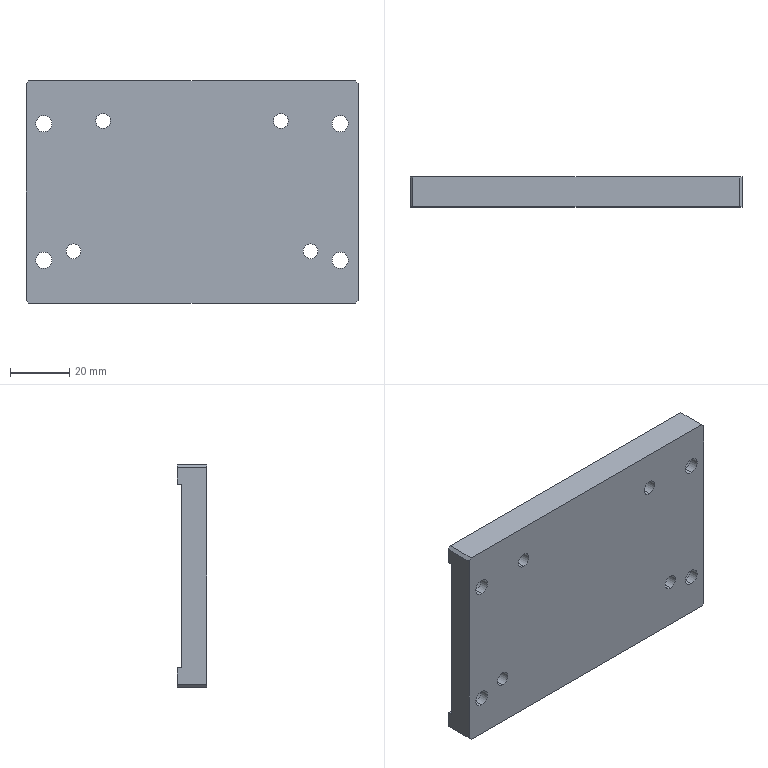Part | NX | features BREP 1 | 1 solid | 42 faces | box 112 x 10 x 75 mm | volume 70883 mm3 | cylinder 24 | plane 18 | commonest cylinder face diameters 5 x8 5.5 x8 10 x8
STEP:
#1=CARTESIAN_POINT('',(-40.,-5.,-22.5));
#2=VERTEX_POINT('',#1);
#3=CARTESIAN_POINT('',(-40.,-5.,-17.5));
#4=VERTEX_POINT('',#3);
#5=CARTESIAN_POINT('',(-40.,-5.,-20.));
#6=DIRECTION('',(0.,1.,0.));
#7=DIRECTION('',(0.,0.,1.));
#8=AXIS2_PLACEMENT_3D('',#5,#6,#7);
#9=CIRCLE('',#8,2.5);
#10=EDGE_CURVE('',#2,#4,#9,.T.);
#11=ORIENTED_EDGE('',*,*,#10,.F.);
#12=CARTESIAN_POINT('',(-40.,3.5,-22.5));
#13=VERTEX_POINT('',#12);
#14=CARTESIAN_POINT('',(-40.,3.5,-22.5));
#15=DIRECTION('',(0.,1.,0.));
#16=VECTOR('',#15,1000.);
#17=LINE('',#14,#16);
#18=EDGE_CURVE('',#13,#2,#17,.F.);
#19=ORIENTED_EDGE('',*,*,#18,.F.);
#20=CARTESIAN_POINT('',(-40.,3.5,-17.5));
#21=VERTEX_POINT('',#20);
#22=CARTESIAN_POINT('',(-40.,3.5,-20.));
#23=DIRECTION('',(0.,1.,0.));
#24=DIRECTION('',(0.,0.,1.));
#25=AXIS2_PLACEMENT_3D('',#22,#23,#24);
#26=CIRCLE('',#25,2.5);
#27=EDGE_CURVE('',#13,#21,#26,.T.);
#28=ORIENTED_EDGE('',*,*,#27,.T.);
#29=CARTESIAN_POINT('',(-40.,3.5,-17.5));
#30=DIRECTION('',(0.,1.,0.));
#31=VECTOR('',#30,1000.);
#32=LINE('',#29,#31);
#33=EDGE_CURVE('',#21,#4,#32,.F.);
#34=ORIENTED_EDGE('',*,*,#33,.T.);
#35=EDGE_LOOP('',(#11,#19,#28,#34));
#36=FACE_BOUND('',#35,.T.);
#37=CARTESIAN_POINT('',(-40.,3.5,-20.));
#38=DIRECTION('',(0.,1.,0.));
#39=DIRECTION('',(0.,0.,1.));
#40=AXIS2_PLACEMENT_3D('',#37,#38,#39);
#41=CYLINDRICAL_SURFACE('',#40,2.5);
#42=ADVANCED_FACE('',(#36),#41,.F.);
#43=CARTESIAN_POINT('',(40.,-5.,-22.5));
#44=VERTEX_POINT('',#43);
#45=CARTESIAN_POINT('',(40.,-5.,-17.5));
#46=VERTEX_POINT('',#45);
#47=CARTESIAN_POINT('',(40.,-5.,-20.));
#48=DIRECTION('',(0.,1.,0.));
#49=DIRECTION('',(0.,0.,1.));
#50=AXIS2_PLACEMENT_3D('',#47,#48,#49);
#51=CIRCLE('',#50,2.5);
#52=EDGE_CURVE('',#44,#46,#51,.T.);
#53=ORIENTED_EDGE('',*,*,#52,.F.);
#54=CARTESIAN_POINT('',(40.,3.5,-22.5));
#55=VERTEX_POINT('',#54);
#56=CARTESIAN_POINT('',(40.,3.5,-22.5));
#57=DIRECTION('',(0.,1.,0.));
#58=VECTOR('',#57,1000.);
#59=LINE('',#56,#58);
#60=EDGE_CURVE('',#55,#44,#59,.F.);
#61=ORIENTED_EDGE('',*,*,#60,.F.);
#62=CARTESIAN_POINT('',(40.,3.5,-17.5));
#63=VERTEX_POINT('',#62);
#64=CARTESIAN_POINT('',(40.,3.5,-20.));
#65=DIRECTION('',(0.,1.,0.));
#66=DIRECTION('',(0.,0.,1.));
#67=AXIS2_PLACEMENT_3D('',#64,#65,#66);
#68=CIRCLE('',#67,2.5);
#69=EDGE_CURVE('',#55,#63,#68,.T.);
#70=ORIENTED_EDGE('',*,*,#69,.T.);
#71=CARTESIAN_POINT('',(40.,3.5,-17.5));
#72=DIRECTION('',(0.,1.,0.));
#73=VECTOR('',#72,1000.);
#74=LINE('',#71,#73);
#75=EDGE_CURVE('',#63,#46,#74,.F.);
#76=ORIENTED_EDGE('',*,*,#75,.T.);
#77=EDGE_LOOP('',(#53,#61,#70,#76));
#78=FACE_BOUND('',#77,.T.);
#79=CARTESIAN_POINT('',(40.,3.5,-20.));
#80=DIRECTION('',(0.,1.,0.));
#81=DIRECTION('',(0.,0.,1.));
#82=AXIS2_PLACEMENT_3D('',#79,#80,#81);
#83=CYLINDRICAL_SURFACE('',#82,2.5);
#84=ADVANCED_FACE('',(#78),#83,.F.);
#85=CARTESIAN_POINT('',(-30.,-5.,21.5));
#86=VERTEX_POINT('',#85);
#87=CARTESIAN_POINT('',(-30.,-5.,26.5));
#88=VERTEX_POINT('',#87);
#89=CARTESIAN_POINT('',(-30.,-5.,24.));
#90=DIRECTION('',(0.,1.,0.));
#91=DIRECTION('',(0.,0.,1.));
#92=AXIS2_PLACEMENT_3D('',#89,#90,#91);
#93=CIRCLE('',#92,2.5);
#94=EDGE_CURVE('',#86,#88,#93,.T.);
#95=ORIENTED_EDGE('',*,*,#94,.F.);
#96=CARTESIAN_POINT('',(-30.,3.5,21.5));
#97=VERTEX_POINT('',#96);
#98=CARTESIAN_POINT('',(-30.,3.5,21.5));
#99=DIRECTION('',(0.,1.,0.));
#100=VECTOR('',#99,1000.);
#101=LINE('',#98,#100);
#102=EDGE_CURVE('',#97,#86,#101,.F.);
#103=ORIENTED_EDGE('',*,*,#102,.F.);
#104=CARTESIAN_POINT('',(-30.,3.5,26.5));
#105=VERTEX_POINT('',#104);
#106=CARTESIAN_POINT('',(-30.,3.5,24.));
#107=DIRECTION('',(0.,1.,0.));
#108=DIRECTION('',(0.,0.,1.));
#109=AXIS2_PLACEMENT_3D('',#106,#107,#108);
#110=CIRCLE('',#109,2.5);
#111=EDGE_CURVE('',#97,#105,#110,.T.);
#112=ORIENTED_EDGE('',*,*,#111,.T.);
#113=CARTESIAN_POINT('',(-30.,3.5,26.5));
#114=DIRECTION('',(0.,1.,0.));
#115=VECTOR('',#114,1000.);
#116=LINE('',#113,#115);
#117=EDGE_CURVE('',#105,#88,#116,.F.);
#118=ORIENTED_EDGE('',*,*,#117,.T.);
#119=EDGE_LOOP('',(#95,#103,#112,#118));
#120=FACE_BOUND('',#119,.T.);
#121=CARTESIAN_POINT('',(-30.,3.5,24.));
#122=DIRECTION('',(0.,1.,0.));
#123=DIRECTION('',(0.,0.,1.));
#124=AXIS2_PLACEMENT_3D('',#121,#122,#123);
#125=CYLINDRICAL_SURFACE('',#124,2.5);
#126=ADVANCED_FACE('',(#120),#125,.F.);
#127=CARTESIAN_POINT('',(30.,-5.,21.5));
#128=VERTEX_POINT('',#127);
#129=CARTESIAN_POINT('',(30.,-5.,26.5));
#130=VERTEX_POINT('',#129);
#131=CARTESIAN_POINT('',(30.,-5.,24.));
#132=DIRECTION('',(0.,1.,0.));
#133=DIRECTION('',(0.,0.,1.));
#134=AXIS2_PLACEMENT_3D('',#131,#132,#133);
#135=CIRCLE('',#134,2.5);
#136=EDGE_CURVE('',#128,#130,#135,.T.);
#137=ORIENTED_EDGE('',*,*,#136,.F.);
#138=CARTESIAN_POINT('',(30.,3.5,21.5));
#139=VERTEX_POINT('',#138);
#140=CARTESIAN_POINT('',(30.,3.5,21.5));
#141=DIRECTION('',(0.,1.,0.));
#142=VECTOR('',#141,1000.);
#143=LINE('',#140,#142);
#144=EDGE_CURVE('',#139,#128,#143,.F.);
#145=ORIENTED_EDGE('',*,*,#144,.F.);
#146=CARTESIAN_POINT('',(30.,3.5,26.5));
#147=VERTEX_POINT('',#146);
#148=CARTESIAN_POINT('',(30.,3.5,24.));
#149=DIRECTION('',(0.,1.,0.));
#150=DIRECTION('',(0.,0.,1.));
#151=AXIS2_PLACEMENT_3D('',#148,#149,#150);
#152=CIRCLE('',#151,2.5);
#153=EDGE_CURVE('',#139,#147,#152,.T.);
#154=ORIENTED_EDGE('',*,*,#153,.T.);
#155=CARTESIAN_POINT('',(30.,3.5,26.5));
#156=DIRECTION('',(0.,1.,0.));
#157=VECTOR('',#156,1000.);
#158=LINE('',#155,#157);
#159=EDGE_CURVE('',#147,#130,#158,.F.);
#160=ORIENTED_EDGE('',*,*,#159,.T.);
#161=EDGE_LOOP('',(#137,#145,#154,#160));
#162=FACE_BOUND('',#161,.T.);
#163=CARTESIAN_POINT('',(30.,3.5,24.));
#164=DIRECTION('',(0.,1.,0.));
#165=DIRECTION('',(0.,0.,1.));
#166=AXIS2_PLACEMENT_3D('',#163,#164,#165);
#167=CYLINDRICAL_SURFACE('',#166,2.5);
#168=ADVANCED_FACE('',(#162),#167,.F.);
#169=CARTESIAN_POINT('',(-50.,-5.,20.25));
#170=VERTEX_POINT('',#169);
#171=CARTESIAN_POINT('',(-50.,-5.,25.75));
#172=VERTEX_POINT('',#171);
#173=CARTESIAN_POINT('',(-50.,-5.,23.));
#174=DIRECTION('',(0.,1.,0.));
#175=DIRECTION('',(0.,0.,1.));
#176=AXIS2_PLACEMENT_3D('',#173,#174,#175);
#177=CIRCLE('',#176,2.75);
#178=EDGE_CURVE('',#170,#172,#177,.T.);
#179=ORIENTED_EDGE('',*,*,#178,.F.);
#180=CARTESIAN_POINT('',(-50.,-2.,20.25));
#181=VERTEX_POINT('',#180);
#182=CARTESIAN_POINT('',(-50.,5.,20.25));
#183=DIRECTION('',(0.,1.,0.));
#184=VECTOR('',#183,1000.);
#185=LINE('',#182,#184);
#186=EDGE_CURVE('',#181,#170,#185,.F.);
#187=ORIENTED_EDGE('',*,*,#186,.F.);
#188=CARTESIAN_POINT('',(-50.,-2.,25.75));
#189=VERTEX_POINT('',#188);
#190=CARTESIAN_POINT('',(-50.,-2.,23.));
#191=DIRECTION('',(0.,1.,0.));
#192=DIRECTION('',(0.,0.,1.));
#193=AXIS2_PLACEMENT_3D('',#190,#191,#192);
#194=CIRCLE('',#193,2.75);
#195=EDGE_CURVE('',#181,#189,#194,.T.);
#196=ORIENTED_EDGE('',*,*,#195,.T.);
#197=CARTESIAN_POINT('',(-50.,5.,25.75));
#198=DIRECTION('',(0.,1.,0.));
#199=VECTOR('',#198,1000.);
#200=LINE('',#197,#199);
#201=EDGE_CURVE('',#189,#172,#200,.F.);
#202=ORIENTED_EDGE('',*,*,#201,.T.);
#203=EDGE_LOOP('',(#179,#187,#196,#202));
#204=FACE_BOUND('',#203,.T.);
#205=CARTESIAN_POINT('',(-50.,5.,23.));
#206=DIRECTION('',(0.,1.,0.));
#207=DIRECTION('',(0.,0.,1.));
#208=AXIS2_PLACEMENT_3D('',#205,#206,#207);
#209=CYLINDRICAL_SURFACE('',#208,2.75);
#210=ADVANCED_FACE('',(#204),#209,.F.);
#211=CARTESIAN_POINT('',(-50.,-5.,-25.75));
#212=VERTEX_POINT('',#211);
#213=CARTESIAN_POINT('',(-50.,-5.,-20.25));
#214=VERTEX_POINT('',#213);
#215=CARTESIAN_POINT('',(-50.,-5.,-23.));
#216=DIRECTION('',(0.,1.,0.));
#217=DIRECTION('',(0.,0.,1.));
#218=AXIS2_PLACEMENT_3D('',#215,#216,#217);
#219=CIRCLE('',#218,2.75);
#220=EDGE_CURVE('',#212,#214,#219,.T.);
#221=ORIENTED_EDGE('',*,*,#220,.F.);
#222=CARTESIAN_POINT('',(-50.,-2.,-25.75));
#223=VERTEX_POINT('',#222);
#224=CARTESIAN_POINT('',(-50.,5.,-25.75));
#225=DIRECTION('',(0.,1.,0.));
#226=VECTOR('',#225,1000.);
#227=LINE('',#224,#226);
#228=EDGE_CURVE('',#223,#212,#227,.F.);
#229=ORIENTED_EDGE('',*,*,#228,.F.);
#230=CARTESIAN_POINT('',(-50.,-2.,-20.25));
#231=VERTEX_POINT('',#230);
#232=CARTESIAN_POINT('',(-50.,-2.,-23.));
#233=DIRECTION('',(0.,1.,0.));
#234=DIRECTION('',(0.,0.,1.));
#235=AXIS2_PLACEMENT_3D('',#232,#233,#234);
#236=CIRCLE('',#235,2.75);
#237=EDGE_CURVE('',#223,#231,#236,.T.);
#238=ORIENTED_EDGE('',*,*,#237,.T.);
#239=CARTESIAN_POINT('',(-50.,5.,-20.25));
#240=DIRECTION('',(0.,1.,0.));
#241=VECTOR('',#240,1000.);
#242=LINE('',#239,#241);
#243=EDGE_CURVE('',#231,#214,#242,.F.);
#244=ORIENTED_EDGE('',*,*,#243,.T.);
#245=EDGE_LOOP('',(#221,#229,#238,#244));
#246=FACE_BOUND('',#245,.T.);
#247=CARTESIAN_POINT('',(-50.,5.,-23.));
#248=DIRECTION('',(0.,1.,0.));
#249=DIRECTION('',(0.,0.,1.));
#250=AXIS2_PLACEMENT_3D('',#247,#248,#249);
#251=CYLINDRICAL_SURFACE('',#250,2.75);
#252=ADVANCED_FACE('',(#246),#251,.F.);
#253=CARTESIAN_POINT('',(50.,-5.,-25.75));
#254=VERTEX_POINT('',#253);
#255=CARTESIAN_POINT('',(50.,-5.,-20.25));
#256=VERTEX_POINT('',#255);
#257=CARTESIAN_POINT('',(50.,-5.,-23.));
#258=DIRECTION('',(0.,1.,0.));
#259=DIRECTION('',(0.,0.,1.));
#260=AXIS2_PLACEMENT_3D('',#257,#258,#259);
#261=CIRCLE('',#260,2.75);
#262=EDGE_CURVE('',#254,#256,#261,.T.);
#263=ORIENTED_EDGE('',*,*,#262,.F.);
#264=CARTESIAN_POINT('',(50.,-2.,-25.75));
#265=VERTEX_POINT('',#264);
#266=CARTESIAN_POINT('',(50.,5.,-25.75));
#267=DIRECTION('',(0.,1.,0.));
#268=VECTOR('',#267,1000.);
#269=LINE('',#266,#268);
#270=EDGE_CURVE('',#265,#254,#269,.F.);
#271=ORIENTED_EDGE('',*,*,#270,.F.);
#272=CARTESIAN_POINT('',(50.,-2.,-20.25));
#273=VERTEX_POINT('',#272);
#274=CARTESIAN_POINT('',(50.,-2.,-23.));
#275=DIRECTION('',(0.,1.,0.));
#276=DIRECTION('',(0.,0.,1.));
#277=AXIS2_PLACEMENT_3D('',#274,#275,#276);
#278=CIRCLE('',#277,2.75);
#279=EDGE_CURVE('',#265,#273,#278,.T.);
#280=ORIENTED_EDGE('',*,*,#279,.T.);
#281=CARTESIAN_POINT('',(50.,5.,-20.25));
#282=DIRECTION('',(0.,1.,0.));
#283=VECTOR('',#282,1000.);
#284=LINE('',#281,#283);
#285=EDGE_CURVE('',#273,#256,#284,.F.);
#286=ORIENTED_EDGE('',*,*,#285,.T.);
#287=EDGE_LOOP('',(#263,#271,#280,#286));
#288=FACE_BOUND('',#287,.T.);
#289=CARTESIAN_POINT('',(50.,5.,-23.));
#290=DIRECTION('',(0.,1.,0.));
#291=DIRECTION('',(0.,0.,1.));
#292=AXIS2_PLACEMENT_3D('',#289,#290,#291);
#293=CYLINDRICAL_SURFACE('',#292,2.75);
#294=ADVANCED_FACE('',(#288),#293,.F.);
#295=CARTESIAN_POINT('',(50.,-5.,20.25));
#296=VERTEX_POINT('',#295);
#297=CARTESIAN_POINT('',(50.,-5.,25.75));
#298=VERTEX_POINT('',#297);
#299=CARTESIAN_POINT('',(50.,-5.,23.));
#300=DIRECTION('',(0.,1.,0.));
#301=DIRECTION('',(0.,0.,1.));
#302=AXIS2_PLACEMENT_3D('',#299,#300,#301);
#303=CIRCLE('',#302,2.75);
#304=EDGE_CURVE('',#296,#298,#303,.T.);
#305=ORIENTED_EDGE('',*,*,#304,.F.);
#306=CARTESIAN_POINT('',(50.,-2.,20.25));
#307=VERTEX_POINT('',#306);
#308=CARTESIAN_POINT('',(50.,5.,20.25));
#309=DIRECTION('',(0.,1.,0.));
#310=VECTOR('',#309,1000.);
#311=LINE('',#308,#310);
#312=EDGE_CURVE('',#307,#296,#311,.F.);
#313=ORIENTED_EDGE('',*,*,#312,.F.);
#314=CARTESIAN_POINT('',(50.,-2.,25.75));
#315=VERTEX_POINT('',#314);
#316=CARTESIAN_POINT('',(50.,-2.,23.));
#317=DIRECTION('',(0.,1.,0.));
#318=DIRECTION('',(0.,0.,1.));
#319=AXIS2_PLACEMENT_3D('',#316,#317,#318);
#320=CIRCLE('',#319,2.75);
#321=EDGE_CURVE('',#307,#315,#320,.T.);
#322=ORIENTED_EDGE('',*,*,#321,.T.);
#323=CARTESIAN_POINT('',(50.,5.,25.75));
#324=DIRECTION('',(0.,1.,0.));
#325=VECTOR('',#324,1000.);
#326=LINE('',#323,#325);
#327=EDGE_CURVE('',#315,#298,#326,.F.);
#328=ORIENTED_EDGE('',*,*,#327,.T.);
#329=EDGE_LOOP('',(#305,#313,#322,#328));
#330=FACE_BOUND('',#329,.T.);
#331=CARTESIAN_POINT('',(50.,5.,23.));
#332=DIRECTION('',(0.,1.,0.));
#333=DIRECTION('',(0.,0.,1.));
#334=AXIS2_PLACEMENT_3D('',#331,#332,#333);
#335=CYLINDRICAL_SURFACE('',#334,2.75);
#336=ADVANCED_FACE('',(#330),#335,.F.);
#337=CARTESIAN_POINT('',(-50.,-2.,18.));
#338=VERTEX_POINT('',#337);
#339=CARTESIAN_POINT('',(-50.,-2.,28.));
#340=VERTEX_POINT('',#339);
#341=CARTESIAN_POINT('',(-50.,-2.,23.));
#342=DIRECTION('',(0.,1.,0.));
#343=DIRECTION('',(0.,0.,1.));
#344=AXIS2_PLACEMENT_3D('',#341,#342,#343);
#345=CIRCLE('',#344,5.);
#346=EDGE_CURVE('',#338,#340,#345,.T.);
#347=ORIENTED_EDGE('',*,*,#346,.F.);
#348=CARTESIAN_POINT('',(-50.,3.5,18.));
#349=VERTEX_POINT('',#348);
#350=CARTESIAN_POINT('',(-50.,5.,18.));
#351=DIRECTION('',(0.,1.,0.));
#352=VECTOR('',#351,1000.);
#353=LINE('',#350,#352);
#354=EDGE_CURVE('',#349,#338,#353,.F.);
#355=ORIENTED_EDGE('',*,*,#354,.F.);
#356=CARTESIAN_POINT('',(-50.,3.5,28.));
#357=VERTEX_POINT('',#356);
#358=CARTESIAN_POINT('',(-50.,3.5,23.));
#359=DIRECTION('',(0.,-1.,0.));
#360=DIRECTION('',(0.,0.,1.));
#361=AXIS2_PLACEMENT_3D('',#358,#359,#360);
#362=CIRCLE('',#361,5.);
#363=EDGE_CURVE('',#357,#349,#362,.T.);
#364=ORIENTED_EDGE('',*,*,#363,.F.);
#365=CARTESIAN_POINT('',(-50.,5.,28.));
#366=DIRECTION('',(0.,1.,0.));
#367=VECTOR('',#366,1000.);
#368=LINE('',#365,#367);
#369=EDGE_CURVE('',#357,#340,#368,.F.);
#370=ORIENTED_EDGE('',*,*,#369,.T.);
#371=EDGE_LOOP('',(#347,#355,#364,#370));
#372=FACE_BOUND('',#371,.T.);
#373=CARTESIAN_POINT('',(-50.,5.,23.));
#374=DIRECTION('',(0.,1.,0.));
#375=DIRECTION('',(0.,0.,1.));
#376=AXIS2_PLACEMENT_3D('',#373,#374,#375);
#377=CYLINDRICAL_SURFACE('',#376,5.);
#378=ADVANCED_FACE('',(#372),#377,.F.);
#379=CARTESIAN_POINT('',(-50.,-2.,-28.));
#380=VERTEX_POINT('',#379);
#381=CARTESIAN_POINT('',(-50.,-2.,-18.));
#382=VERTEX_POINT('',#381);
#383=CARTESIAN_POINT('',(-50.,-2.,-23.));
#384=DIRECTION('',(0.,1.,0.));
#385=DIRECTION('',(0.,0.,1.));
#386=AXIS2_PLACEMENT_3D('',#383,#384,#385);
#387=CIRCLE('',#386,5.);
#388=EDGE_CURVE('',#380,#382,#387,.T.);
#389=ORIENTED_EDGE('',*,*,#388,.F.);
#390=CARTESIAN_POINT('',(-50.,3.5,-28.));
#391=VERTEX_POINT('',#390);
#392=CARTESIAN_POINT('',(-50.,5.,-28.));
#393=DIRECTION('',(0.,1.,0.));
#394=VECTOR('',#393,1000.);
#395=LINE('',#392,#394);
#396=EDGE_CURVE('',#391,#380,#395,.F.);
#397=ORIENTED_EDGE('',*,*,#396,.F.);
#398=CARTESIAN_POINT('',(-50.,3.5,-18.));
#399=VERTEX_POINT('',#398);
#400=CARTESIAN_POINT('',(-50.,3.5,-23.));
#401=DIRECTION('',(0.,-1.,0.));
#402=DIRECTION('',(0.,0.,1.));
#403=AXIS2_PLACEMENT_3D('',#400,#401,#402);
#404=CIRCLE('',#403,5.);
#405=EDGE_CURVE('',#399,#391,#404,.T.);
#406=ORIENTED_EDGE('',*,*,#405,.F.);
#407=CARTESIAN_POINT('',(-50.,5.,-18.));
#408=DIRECTION('',(0.,1.,0.));
#409=VECTOR('',#408,1000.);
#410=LINE('',#407,#409);
#411=EDGE_CURVE('',#399,#382,#410,.F.);
#412=ORIENTED_EDGE('',*,*,#411,.T.);
#413=EDGE_LOOP('',(#389,#397,#406,#412));
#414=FACE_BOUND('',#413,.T.);
#415=CARTESIAN_POINT('',(-50.,5.,-23.));
#416=DIRECTION('',(0.,1.,0.));
#417=DIRECTION('',(0.,0.,1.));
#418=AXIS2_PLACEMENT_3D('',#415,#416,#417);
#419=CYLINDRICAL_SURFACE('',#418,5.);
#420=ADVANCED_FACE('',(#414),#419,.F.);
#421=CARTESIAN_POINT('',(50.,-2.,-28.));
#422=VERTEX_POINT('',#421);
#423=CARTESIAN_POINT('',(50.,-2.,-18.));
#424=VERTEX_POINT('',#423);
#425=CARTESIAN_POINT('',(50.,-2.,-23.));
#426=DIRECTION('',(0.,1.,0.));
#427=DIRECTION('',(0.,0.,1.));
#428=AXIS2_PLACEMENT_3D('',#425,#426,#427);
#429=CIRCLE('',#428,5.);
#430=EDGE_CURVE('',#422,#424,#429,.T.);
#431=ORIENTED_EDGE('',*,*,#430,.F.);
#432=CARTESIAN_POINT('',(50.,3.5,-28.));
#433=VERTEX_POINT('',#432);
#434=CARTESIAN_POINT('',(50.,5.,-28.));
#435=DIRECTION('',(0.,1.,0.));
#436=VECTOR('',#435,1000.);
#437=LINE('',#434,#436);
#438=EDGE_CURVE('',#433,#422,#437,.F.);
#439=ORIENTED_EDGE('',*,*,#438,.F.);
#440=CARTESIAN_POINT('',(50.,3.5,-18.));
#441=VERTEX_POINT('',#440);
#442=CARTESIAN_POINT('',(50.,3.5,-23.));
#443=DIRECTION('',(0.,-1.,0.));
#444=DIRECTION('',(0.,0.,1.));
#445=AXIS2_PLACEMENT_3D('',#442,#443,#444);
#446=CIRCLE('',#445,5.);
#447=EDGE_CURVE('',#441,#433,#446,.T.);
#448=ORIENTED_EDGE('',*,*,#447,.F.);
#449=CARTESIAN_POINT('',(50.,5.,-18.));
#450=DIRECTION('',(0.,1.,0.));
#451=VECTOR('',#450,1000.);
#452=LINE('',#449,#451);
#453=EDGE_CURVE('',#441,#424,#452,.F.);
#454=ORIENTED_EDGE('',*,*,#453,.T.);
#455=EDGE_LOOP('',(#431,#439,#448,#454));
#456=FACE_BOUND('',#455,.T.);
#457=CARTESIAN_POINT('',(50.,5.,-23.));
#458=DIRECTION('',(0.,1.,0.));
#459=DIRECTION('',(0.,0.,1.));
#460=AXIS2_PLACEMENT_3D('',#457,#458,#459);
#461=CYLINDRICAL_SURFACE('',#460,5.);
#462=ADVANCED_FACE('',(#456),#461,.F.);
#463=CARTESIAN_POINT('',(50.,-2.,18.));
#464=VERTEX_POINT('',#463);
#465=CARTESIAN_POINT('',(50.,-2.,28.));
#466=VERTEX_POINT('',#465);
#467=CARTESIAN_POINT('',(50.,-2.,23.));
#468=DIRECTION('',(0.,1.,0.));
#469=DIRECTION('',(0.,0.,1.));
#470=AXIS2_PLACEMENT_3D('',#467,#468,#469);
#471=CIRCLE('',#470,5.);
#472=EDGE_CURVE('',#464,#466,#471,.T.);
#473=ORIENTED_EDGE('',*,*,#472,.F.);
#474=CARTESIAN_POINT('',(50.,3.5,18.));
#475=VERTEX_POINT('',#474);
#476=CARTESIAN_POINT('',(50.,5.,18.));
#477=DIRECTION('',(0.,1.,0.));
#478=VECTOR('',#477,1000.);
#479=LINE('',#476,#478);
#480=EDGE_CURVE('',#475,#464,#479,.F.);
#481=ORIENTED_EDGE('',*,*,#480,.F.);
#482=CARTESIAN_POINT('',(50.,3.5,28.));
#483=VERTEX_POINT('',#482);
#484=CARTESIAN_POINT('',(50.,3.5,23.));
#485=DIRECTION('',(0.,-1.,0.));
#486=DIRECTION('',(0.,0.,1.));
#487=AXIS2_PLACEMENT_3D('',#484,#485,#486);
#488=CIRCLE('',#487,5.);
#489=EDGE_CURVE('',#483,#475,#488,.T.);
#490=ORIENTED_EDGE('',*,*,#489,.F.);
#491=CARTESIAN_POINT('',(50.,5.,28.));
#492=DIRECTION('',(0.,1.,0.));
#493=VECTOR('',#492,1000.);
#494=LINE('',#491,#493);
#495=EDGE_CURVE('',#483,#466,#494,.F.);
#496=ORIENTED_EDGE('',*,*,#495,.T.);
#497=EDGE_LOOP('',(#473,#481,#490,#496));
#498=FACE_BOUND('',#497,.T.);
#499=CARTESIAN_POINT('',(50.,5.,23.));
#500=DIRECTION('',(0.,1.,0.));
#501=DIRECTION('',(0.,0.,1.));
#502=AXIS2_PLACEMENT_3D('',#499,#500,#501);
#503=CYLINDRICAL_SURFACE('',#502,5.);
#504=ADVANCED_FACE('',(#498),#503,.F.);
#505=CARTESIAN_POINT('',(-56.,5.,31.));
#506=VERTEX_POINT('',#505);
#507=CARTESIAN_POINT('',(56.,5.,31.));
#508=VERTEX_POINT('',#507);
#509=CARTESIAN_POINT('',(56.,5.,31.));
#510=DIRECTION('',(1.,0.,0.));
#511=VECTOR('',#510,1000.);
#512=LINE('',#509,#511);
#513=EDGE_CURVE('',#506,#508,#512,.T.);
#514=ORIENTED_EDGE('',*,*,#513,.F.);
#515=CARTESIAN_POINT('',(-56.,5.,36.5));
#516=VERTEX_POINT('',#515);
#517=CARTESIAN_POINT('',(-56.,5.,-37.5));
#518=DIRECTION('',(0.,0.,1.));
#519=VECTOR('',#518,1000.);
#520=LINE('',#517,#519);
#521=EDGE_CURVE('',#506,#516,#520,.T.);
#522=ORIENTED_EDGE('',*,*,#521,.T.);
#523=CARTESIAN_POINT('',(-55.,5.,37.5));
#524=VERTEX_POINT('',#523);
#525=CARTESIAN_POINT('',(-46.25,5.,46.25));
#526=DIRECTION('',(0.7071,0.,0.7071));
#527=VECTOR('',#526,1000.);
#528=LINE('',#525,#527);
#529=EDGE_CURVE('',#516,#524,#528,.T.);
#530=ORIENTED_EDGE('',*,*,#529,.T.);
#531=CARTESIAN_POINT('',(55.,5.,37.5));
#532=VERTEX_POINT('',#531);
#533=CARTESIAN_POINT('',(-56.,5.,37.5));
#534=DIRECTION('',(1.,0.,0.));
#535=VECTOR('',#534,1000.);
#536=LINE('',#533,#535);
#537=EDGE_CURVE('',#524,#532,#536,.T.);
#538=ORIENTED_EDGE('',*,*,#537,.T.);
#539=CARTESIAN_POINT('',(56.,5.,36.5));
#540=VERTEX_POINT('',#539);
#541=CARTESIAN_POINT('',(46.25,5.,46.25));
#542=DIRECTION('',(0.7071,0.,-0.7071));
#543=VECTOR('',#542,1000.);
#544=LINE('',#541,#543);
#545=EDGE_CURVE('',#532,#540,#544,.T.);
#546=ORIENTED_EDGE('',*,*,#545,.T.);
#547=CARTESIAN_POINT('',(56.,5.,-37.5));
#548=DIRECTION('',(0.,0.,-1.));
#549=VECTOR('',#548,1000.);
#550=LINE('',#547,#549);
#551=EDGE_CURVE('',#540,#508,#550,.T.);
#552=ORIENTED_EDGE('',*,*,#551,.T.);
#553=EDGE_LOOP('',(#514,#522,#530,#538,#546,#552));
#554=FACE_BOUND('',#553,.T.);
#555=CARTESIAN_POINT('',(0.,5.,0.));
#556=DIRECTION('',(0.,1.,0.));
#557=DIRECTION('',(1.,0.,0.));
#558=AXIS2_PLACEMENT_3D('',#555,#556,#557);
#559=PLANE('',#558);
#560=ADVANCED_FACE('',(#554),#559,.T.);
#561=ORIENTED_EDGE('',*,*,#480,.T.);
#562=CARTESIAN_POINT('',(50.,-2.,23.));
#563=DIRECTION('',(0.,1.,0.));
#564=DIRECTION('',(0.,0.,1.));
#565=AXIS2_PLACEMENT_3D('',#562,#563,#564);
#566=CIRCLE('',#565,5.);
#567=EDGE_CURVE('',#466,#464,#566,.T.);
#568=ORIENTED_EDGE('',*,*,#567,.F.);
#569=ORIENTED_EDGE('',*,*,#495,.F.);
#570=CARTESIAN_POINT('',(50.,3.5,23.));
#571=DIRECTION('',(0.,-1.,0.));
#572=DIRECTION('',(0.,0.,1.));
#573=AXIS2_PLACEMENT_3D('',#570,#571,#572);
#574=CIRCLE('',#573,5.);
#575=EDGE_CURVE('',#475,#483,#574,.T.);
#576=ORIENTED_EDGE('',*,*,#575,.F.);
#577=EDGE_LOOP('',(#561,#568,#569,#576));
#578=FACE_BOUND('',#577,.T.);
#579=CARTESIAN_POINT('',(50.,5.,23.));
#580=DIRECTION('',(0.,1.,0.));
#581=DIRECTION('',(0.,0.,1.));
#582=AXIS2_PLACEMENT_3D('',#579,#580,#581);
#583=CYLINDRICAL_SURFACE('',#582,5.);
#584=ADVANCED_FACE('',(#578),#583,.F.);
#585=ORIENTED_EDGE('',*,*,#438,.T.);
#586=CARTESIAN_POINT('',(50.,-2.,-23.));
#587=DIRECTION('',(0.,1.,0.));
#588=DIRECTION('',(0.,0.,1.));
#589=AXIS2_PLACEMENT_3D('',#586,#587,#588);
#590=CIRCLE('',#589,5.);
#591=EDGE_CURVE('',#424,#422,#590,.T.);
#592=ORIENTED_EDGE('',*,*,#591,.F.);
#593=ORIENTED_EDGE('',*,*,#453,.F.);
#594=CARTESIAN_POINT('',(50.,3.5,-23.));
#595=DIRECTION('',(0.,-1.,0.));
#596=DIRECTION('',(0.,0.,1.));
#597=AXIS2_PLACEMENT_3D('',#594,#595,#596);
#598=CIRCLE('',#597,5.);
#599=EDGE_CURVE('',#433,#441,#598,.T.);
#600=ORIENTED_EDGE('',*,*,#599,.F.);
#601=EDGE_LOOP('',(#585,#592,#593,#600));
#602=FACE_BOUND('',#601,.T.);
#603=CARTESIAN_POINT('',(50.,5.,-23.));
#604=DIRECTION('',(0.,1.,0.));
#605=DIRECTION('',(0.,0.,1.));
#606=AXIS2_PLACEMENT_3D('',#603,#604,#605);
#607=CYLINDRICAL_SURFACE('',#606,5.);
#608=ADVANCED_FACE('',(#602),#607,.F.);
#609=ORIENTED_EDGE('',*,*,#396,.T.);
#610=CARTESIAN_POINT('',(-50.,-2.,-23.));
#611=DIRECTION('',(0.,1.,0.));
#612=DIRECTION('',(0.,0.,1.));
#613=AXIS2_PLACEMENT_3D('',#610,#611,#612);
#614=CIRCLE('',#613,5.);
#615=EDGE_CURVE('',#382,#380,#614,.T.);
#616=ORIENTED_EDGE('',*,*,#615,.F.);
#617=ORIENTED_EDGE('',*,*,#411,.F.);
#618=CARTESIAN_POINT('',(-50.,3.5,-23.));
#619=DIRECTION('',(0.,-1.,0.));
#620=DIRECTION('',(0.,0.,1.));
#621=AXIS2_PLACEMENT_3D('',#618,#619,#620);
#622=CIRCLE('',#621,5.);
#623=EDGE_CURVE('',#391,#399,#622,.T.);
#624=ORIENTED_EDGE('',*,*,#623,.F.);
#625=EDGE_LOOP('',(#609,#616,#617,#624));
#626=FACE_BOUND('',#625,.T.);
#627=CARTESIAN_POINT('',(-50.,5.,-23.));
#628=DIRECTION('',(0.,1.,0.));
#629=DIRECTION('',(0.,0.,1.));
#630=AXIS2_PLACEMENT_3D('',#627,#628,#629);
#631=CYLINDRICAL_SURFACE('',#630,5.);
#632=ADVANCED_FACE('',(#626),#631,.F.);
#633=ORIENTED_EDGE('',*,*,#354,.T.);
#634=CARTESIAN_POINT('',(-50.,-2.,23.));
#635=DIRECTION('',(0.,1.,0.));
#636=DIRECTION('',(0.,0.,1.));
#637=AXIS2_PLACEMENT_3D('',#634,#635,#636);
#638=CIRCLE('',#637,5.);
#639=EDGE_CURVE('',#340,#338,#638,.T.);
#640=ORIENTED_EDGE('',*,*,#639,.F.);
#641=ORIENTED_EDGE('',*,*,#369,.F.);
#642=CARTESIAN_POINT('',(-50.,3.5,23.));
#643=DIRECTION('',(0.,-1.,0.));
#644=DIRECTION('',(0.,0.,1.));
#645=AXIS2_PLACEMENT_3D('',#642,#643,#644);
#646=CIRCLE('',#645,5.);
#647=EDGE_CURVE('',#349,#357,#646,.T.);
#648=ORIENTED_EDGE('',*,*,#647,.F.);
#649=EDGE_LOOP('',(#633,#640,#641,#648));
#650=FACE_BOUND('',#649,.T.);
#651=CARTESIAN_POINT('',(-50.,5.,23.));
#652=DIRECTION('',(0.,1.,0.));
#653=DIRECTION('',(0.,0.,1.));
#654=AXIS2_PLACEMENT_3D('',#651,#652,#653);
#655=CYLINDRICAL_SURFACE('',#654,5.);
#656=ADVANCED_FACE('',(#650),#655,.F.);
#657=CARTESIAN_POINT('',(56.,3.5,31.));
#658=VERTEX_POINT('',#657);
#659=CARTESIAN_POINT('',(56.,3.5,-31.));
#660=VERTEX_POINT('',#659);
#661=CARTESIAN_POINT('',(56.,3.5,31.));
#662=DIRECTION('',(0.,0.,-1.));
#663=VECTOR('',#662,1000.);
#664=LINE('',#661,#663);
#665=EDGE_CURVE('',#658,#660,#664,.T.);
#666=ORIENTED_EDGE('',*,*,#665,.F.);
#667=CARTESIAN_POINT('',(56.,3.5,31.));
#668=DIRECTION('',(0.,1.,0.));
#669=VECTOR('',#668,1000.);
#670=LINE('',#667,#669);
#671=EDGE_CURVE('',#658,#508,#670,.T.);
#672=ORIENTED_EDGE('',*,*,#671,.T.);
#673=ORIENTED_EDGE('',*,*,#551,.F.);
#674=CARTESIAN_POINT('',(56.,-5.,36.5));
#675=VERTEX_POINT('',#674);
#676=CARTESIAN_POINT('',(56.,5.,36.5));
#677=DIRECTION('',(0.,-1.,0.));
#678=VECTOR('',#677,1000.);
#679=LINE('',#676,#678);
#680=EDGE_CURVE('',#540,#675,#679,.T.);
#681=ORIENTED_EDGE('',*,*,#680,.T.);
#682=CARTESIAN_POINT('',(56.,-5.,-36.5));
#683=VERTEX_POINT('',#682);
#684=CARTESIAN_POINT('',(56.,-5.,-37.5));
#685=DIRECTION('',(0.,0.,-1.));
#686=VECTOR('',#685,1000.);
#687=LINE('',#684,#686);
#688=EDGE_CURVE('',#675,#683,#687,.T.);
#689=ORIENTED_EDGE('',*,*,#688,.T.);
#690=CARTESIAN_POINT('',(56.,5.,-36.5));
#691=VERTEX_POINT('',#690);
#692=CARTESIAN_POINT('',(56.,5.,-36.5));
#693=DIRECTION('',(0.,1.,0.));
#694=VECTOR('',#693,1000.);
#695=LINE('',#692,#694);
#696=EDGE_CURVE('',#683,#691,#695,.T.);
#697=ORIENTED_EDGE('',*,*,#696,.T.);
#698=CARTESIAN_POINT('',(56.,5.,-31.));
#699=VERTEX_POINT('',#698);
#700=CARTESIAN_POINT('',(56.,5.,-37.5));
#701=DIRECTION('',(0.,0.,-1.));
#702=VECTOR('',#701,1000.);
#703=LINE('',#700,#702);
#704=EDGE_CURVE('',#699,#691,#703,.T.);
#705=ORIENTED_EDGE('',*,*,#704,.F.);
#706=CARTESIAN_POINT('',(56.,3.5,-31.));
#707=DIRECTION('',(0.,1.,0.));
#708=VECTOR('',#707,1000.);
#709=LINE('',#706,#708);
#710=EDGE_CURVE('',#660,#699,#709,.T.);
#711=ORIENTED_EDGE('',*,*,#710,.F.);
#712=EDGE_LOOP('',(#666,#672,#673,#681,#689,#697,#705,#711));
#713=FACE_BOUND('',#712,.T.);
#714=CARTESIAN_POINT('',(56.,5.,-37.5));
#715=DIRECTION('',(-1.,0.,0.));
#716=DIRECTION('',(0.,0.,1.));
#717=AXIS2_PLACEMENT_3D('',#714,#715,#716);
#718=PLANE('',#717);
#719=ADVANCED_FACE('',(#713),#718,.F.);
#720=CARTESIAN_POINT('',(55.,-5.,-37.5));
#721=VERTEX_POINT('',#720);
#722=CARTESIAN_POINT('',(-55.,-5.,-37.5));
#723=VERTEX_POINT('',#722);
#724=CARTESIAN_POINT('',(-56.,-5.,-37.5));
#725=DIRECTION('',(-1.,0.,0.));
#726=VECTOR('',#725,1000.);
#727=LINE('',#724,#726);
#728=EDGE_CURVE('',#721,#723,#727,.T.);
#729=ORIENTED_EDGE('',*,*,#728,.T.);
#730=CARTESIAN_POINT('',(-55.,5.,-37.5));
#731=VERTEX_POINT('',#730);
#732=CARTESIAN_POINT('',(-55.,5.,-37.5));
#733=DIRECTION('',(0.,1.,0.));
#734=VECTOR('',#733,1000.);
#735=LINE('',#732,#734);
#736=EDGE_CURVE('',#723,#731,#735,.T.);
#737=ORIENTED_EDGE('',*,*,#736,.T.);
#738=CARTESIAN_POINT('',(55.,5.,-37.5));
#739=VERTEX_POINT('',#738);
#740=CARTESIAN_POINT('',(-56.,5.,-37.5));
#741=DIRECTION('',(-1.,0.,0.));
#742=VECTOR('',#741,1000.);
#743=LINE('',#740,#742);
#744=EDGE_CURVE('',#739,#731,#743,.T.);
#745=ORIENTED_EDGE('',*,*,#744,.F.);
#746=CARTESIAN_POINT('',(55.,5.,-37.5));
#747=DIRECTION('',(0.,-1.,0.));
#748=VECTOR('',#747,1000.);
#749=LINE('',#746,#748);
#750=EDGE_CURVE('',#739,#721,#749,.T.);
#751=ORIENTED_EDGE('',*,*,#750,.T.);
#752=EDGE_LOOP('',(#729,#737,#745,#751));
#753=FACE_BOUND('',#752,.T.);
#754=CARTESIAN_POINT('',(-56.,5.,-37.5));
#755=DIRECTION('',(0.,0.,1.));
#756=DIRECTION('',(1.,0.,0.));
#757=AXIS2_PLACEMENT_3D('',#754,#755,#756);
#758=PLANE('',#757);
#759=ADVANCED_FACE('',(#753),#758,.F.);
#760=ORIENTED_EDGE('',*,*,#521,.F.);
#761=CARTESIAN_POINT('',(-56.,3.5,31.));
#762=VERTEX_POINT('',#761);
#763=CARTESIAN_POINT('',(-56.,3.5,31.));
#764=DIRECTION('',(0.,1.,0.));
#765=VECTOR('',#764,1000.);
#766=LINE('',#763,#765);
#767=EDGE_CURVE('',#762,#506,#766,.T.);
#768=ORIENTED_EDGE('',*,*,#767,.F.);
#769=CARTESIAN_POINT('',(-56.,3.5,-31.));
#770=VERTEX_POINT('',#769);
#771=CARTESIAN_POINT('',(-56.,3.5,31.));
#772=DIRECTION('',(0.,0.,1.));
#773=VECTOR('',#772,1000.);
#774=LINE('',#771,#773);
#775=EDGE_CURVE('',#770,#762,#774,.T.);
#776=ORIENTED_EDGE('',*,*,#775,.F.);
#777=CARTESIAN_POINT('',(-56.,5.,-31.));
#778=VERTEX_POINT('',#777);
#779=CARTESIAN_POINT('',(-56.,3.5,-31.));
#780=DIRECTION('',(0.,1.,0.));
#781=VECTOR('',#780,1000.);
#782=LINE('',#779,#781);
#783=EDGE_CURVE('',#770,#778,#782,.T.);
#784=ORIENTED_EDGE('',*,*,#783,.T.);
#785=CARTESIAN_POINT('',(-56.,5.,-36.5));
#786=VERTEX_POINT('',#785);
#787=CARTESIAN_POINT('',(-56.,5.,-37.5));
#788=DIRECTION('',(0.,0.,1.));
#789=VECTOR('',#788,1000.);
#790=LINE('',#787,#789);
#791=EDGE_CURVE('',#786,#778,#790,.T.);
#792=ORIENTED_EDGE('',*,*,#791,.F.);
#793=CARTESIAN_POINT('',(-56.,-5.,-36.5));
#794=VERTEX_POINT('',#793);
#795=CARTESIAN_POINT('',(-56.,5.,-36.5));
#796=DIRECTION('',(0.,-1.,0.));
#797=VECTOR('',#796,1000.);
#798=LINE('',#795,#797);
#799=EDGE_CURVE('',#786,#794,#798,.T.);
#800=ORIENTED_EDGE('',*,*,#799,.T.);
#801=CARTESIAN_POINT('',(-56.,-5.,36.5));
#802=VERTEX_POINT('',#801);
#803=CARTESIAN_POINT('',(-56.,-5.,-37.5));
#804=DIRECTION('',(0.,0.,1.));
#805=VECTOR('',#804,1000.);
#806=LINE('',#803,#805);
#807=EDGE_CURVE('',#794,#802,#806,.T.);
#808=ORIENTED_EDGE('',*,*,#807,.T.);
#809=CARTESIAN_POINT('',(-56.,5.,36.5));
#810=DIRECTION('',(0.,1.,0.));
#811=VECTOR('',#810,1000.);
#812=LINE('',#809,#811);
#813=EDGE_CURVE('',#802,#516,#812,.T.);
#814=ORIENTED_EDGE('',*,*,#813,.T.);
#815=EDGE_LOOP('',(#760,#768,#776,#784,#792,#800,#808,#814));
#816=FACE_BOUND('',#815,.T.);
#817=CARTESIAN_POINT('',(-56.,5.,-37.5));
#818=DIRECTION('',(1.,0.,0.));
#819=DIRECTION('',(0.,0.,-1.));
#820=AXIS2_PLACEMENT_3D('',#817,#818,#819);
#821=PLANE('',#820);
#822=ADVANCED_FACE('',(#816),#821,.F.);
#823=ORIENTED_EDGE('',*,*,#537,.F.);
#824=CARTESIAN_POINT('',(-55.,-5.,37.5));
#825=VERTEX_POINT('',#824);
#826=CARTESIAN_POINT('',(-55.,5.,37.5));
#827=DIRECTION('',(0.,-1.,0.));
#828=VECTOR('',#827,1000.);
#829=LINE('',#826,#828);
#830=EDGE_CURVE('',#524,#825,#829,.T.);
#831=ORIENTED_EDGE('',*,*,#830,.T.);
#832=CARTESIAN_POINT('',(55.,-5.,37.5));
#833=VERTEX_POINT('',#832);
#834=CARTESIAN_POINT('',(-56.,-5.,37.5));
#835=DIRECTION('',(1.,0.,0.));
#836=VECTOR('',#835,1000.);
#837=LINE('',#834,#836);
#838=EDGE_CURVE('',#825,#833,#837,.T.);
#839=ORIENTED_EDGE('',*,*,#838,.T.);
#840=CARTESIAN_POINT('',(55.,5.,37.5));
#841=DIRECTION('',(0.,1.,0.));
#842=VECTOR('',#841,1000.);
#843=LINE('',#840,#842);
#844=EDGE_CURVE('',#833,#532,#843,.T.);
#845=ORIENTED_EDGE('',*,*,#844,.T.);
#846=EDGE_LOOP('',(#823,#831,#839,#845));
#847=FACE_BOUND('',#846,.T.);
#848=CARTESIAN_POINT('',(-56.,5.,37.5));
#849=DIRECTION('',(0.,0.,-1.));
#850=DIRECTION('',(0.,-1.,0.));
#851=AXIS2_PLACEMENT_3D('',#848,#849,#850);
#852=PLANE('',#851);
#853=ADVANCED_FACE('',(#847),#852,.F.);
#854=CARTESIAN_POINT('',(56.,5.,-31.));
#855=DIRECTION('',(-1.,0.,0.));
#856=VECTOR('',#855,1000.);
#857=LINE('',#854,#856);
#858=EDGE_CURVE('',#699,#778,#857,.T.);
#859=ORIENTED_EDGE('',*,*,#858,.F.);
#860=ORIENTED_EDGE('',*,*,#704,.T.);
#861=CARTESIAN_POINT('',(46.25,5.,-46.25));
#862=DIRECTION('',(-0.7071,0.,-0.7071));
#863=VECTOR('',#862,1000.);
#864=LINE('',#861,#863);
#865=EDGE_CURVE('',#691,#739,#864,.T.);
#866=ORIENTED_EDGE('',*,*,#865,.T.);
#867=ORIENTED_EDGE('',*,*,#744,.T.);
#868=CARTESIAN_POINT('',(-46.25,5.,-46.25));
#869=DIRECTION('',(-0.7071,0.,0.7071));
#870=VECTOR('',#869,1000.);
#871=LINE('',#868,#870);
#872=EDGE_CURVE('',#731,#786,#871,.T.);
#873=ORIENTED_EDGE('',*,*,#872,.T.);
#874=ORIENTED_EDGE('',*,*,#791,.T.);
#875=EDGE_LOOP('',(#859,#860,#866,#867,#873,#874));
#876=FACE_BOUND('',#875,.T.);
#877=CARTESIAN_POINT('',(0.,5.,0.));
#878=DIRECTION('',(0.,1.,0.));
#879=DIRECTION('',(1.,0.,0.));
#880=AXIS2_PLACEMENT_3D('',#877,#878,#879);
#881=PLANE('',#880);
#882=ADVANCED_FACE('',(#876),#881,.T.);
#883=ORIENTED_EDGE('',*,*,#807,.F.);
#884=CARTESIAN_POINT('',(-56.,-5.,-36.5));
#885=DIRECTION('',(0.7071,0.,-0.7071));
#886=VECTOR('',#885,1000.);
#887=LINE('',#884,#886);
#888=EDGE_CURVE('',#794,#723,#887,.T.);
#889=ORIENTED_EDGE('',*,*,#888,.T.);
#890=ORIENTED_EDGE('',*,*,#728,.F.);
#891=CARTESIAN_POINT('',(55.,-5.,-37.5));
#892=DIRECTION('',(0.7071,0.,0.7071));
#893=VECTOR('',#892,1000.);
#894=LINE('',#891,#893);
#895=EDGE_CURVE('',#721,#683,#894,.T.);
#896=ORIENTED_EDGE('',*,*,#895,.T.);
#897=ORIENTED_EDGE('',*,*,#688,.F.);
#898=CARTESIAN_POINT('',(56.,-5.,36.5));
#899=DIRECTION('',(-0.7071,0.,0.7071));
#900=VECTOR('',#899,1000.);
#901=LINE('',#898,#900);
#902=EDGE_CURVE('',#675,#833,#901,.T.);
#903=ORIENTED_EDGE('',*,*,#902,.T.);
#904=ORIENTED_EDGE('',*,*,#838,.F.);
#905=CARTESIAN_POINT('',(-55.,-5.,37.5));
#906=DIRECTION('',(-0.7071,0.,-0.7071));
#907=VECTOR('',#906,1000.);
#908=LINE('',#905,#907);
#909=EDGE_CURVE('',#825,#802,#908,.T.);
#910=ORIENTED_EDGE('',*,*,#909,.T.);
#911=EDGE_LOOP('',(#883,#889,#890,#896,#897,#903,#904,#910));
#912=FACE_BOUND('',#911,.T.);
#913=CARTESIAN_POINT('',(-40.,-5.,-20.));
#914=DIRECTION('',(0.,1.,0.));
#915=DIRECTION('',(0.,0.,1.));
#916=AXIS2_PLACEMENT_3D('',#913,#914,#915);
#917=CIRCLE('',#916,2.5);
#918=EDGE_CURVE('',#4,#2,#917,.T.);
#919=ORIENTED_EDGE('',*,*,#918,.T.);
#920=ORIENTED_EDGE('',*,*,#10,.T.);
#921=EDGE_LOOP('',(#919,#920));
#922=FACE_BOUND('',#921,.T.);
#923=CARTESIAN_POINT('',(40.,-5.,-20.));
#924=DIRECTION('',(0.,1.,0.));
#925=DIRECTION('',(0.,0.,1.));
#926=AXIS2_PLACEMENT_3D('',#923,#924,#925);
#927=CIRCLE('',#926,2.5);
#928=EDGE_CURVE('',#46,#44,#927,.T.);
#929=ORIENTED_EDGE('',*,*,#928,.T.);
#930=ORIENTED_EDGE('',*,*,#52,.T.);
#931=EDGE_LOOP('',(#929,#930));
#932=FACE_BOUND('',#931,.T.);
#933=CARTESIAN_POINT('',(-30.,-5.,24.));
#934=DIRECTION('',(0.,1.,0.));
#935=DIRECTION('',(0.,0.,1.));
#936=AXIS2_PLACEMENT_3D('',#933,#934,#935);
#937=CIRCLE('',#936,2.5);
#938=EDGE_CURVE('',#88,#86,#937,.T.);
#939=ORIENTED_EDGE('',*,*,#938,.T.);
#940=ORIENTED_EDGE('',*,*,#94,.T.);
#941=EDGE_LOOP('',(#939,#940));
#942=FACE_BOUND('',#941,.T.);
#943=CARTESIAN_POINT('',(30.,-5.,24.));
#944=DIRECTION('',(0.,1.,0.));
#945=DIRECTION('',(0.,0.,1.));
#946=AXIS2_PLACEMENT_3D('',#943,#944,#945);
#947=CIRCLE('',#946,2.5);
#948=EDGE_CURVE('',#130,#128,#947,.T.);
#949=ORIENTED_EDGE('',*,*,#948,.T.);
#950=ORIENTED_EDGE('',*,*,#136,.T.);
#951=EDGE_LOOP('',(#949,#950));
#952=FACE_BOUND('',#951,.T.);
#953=CARTESIAN_POINT('',(-50.,-5.,23.));
#954=DIRECTION('',(0.,1.,0.));
#955=DIRECTION('',(0.,0.,1.));
#956=AXIS2_PLACEMENT_3D('',#953,#954,#955);
#957=CIRCLE('',#956,2.75);
#958=EDGE_CURVE('',#172,#170,#957,.T.);
#959=ORIENTED_EDGE('',*,*,#958,.T.);
#960=ORIENTED_EDGE('',*,*,#178,.T.);
#961=EDGE_LOOP('',(#959,#960));
#962=FACE_BOUND('',#961,.T.);
#963=CARTESIAN_POINT('',(-50.,-5.,-23.));
#964=DIRECTION('',(0.,1.,0.));
#965=DIRECTION('',(0.,0.,1.));
#966=AXIS2_PLACEMENT_3D('',#963,#964,#965);
#967=CIRCLE('',#966,2.75);
#968=EDGE_CURVE('',#214,#212,#967,.T.);
#969=ORIENTED_EDGE('',*,*,#968,.T.);
#970=ORIENTED_EDGE('',*,*,#220,.T.);
#971=EDGE_LOOP('',(#969,#970));
#972=FACE_BOUND('',#971,.T.);
#973=CARTESIAN_POINT('',(50.,-5.,-23.));
#974=DIRECTION('',(0.,1.,0.));
#975=DIRECTION('',(0.,0.,1.));
#976=AXIS2_PLACEMENT_3D('',#973,#974,#975);
#977=CIRCLE('',#976,2.75);
#978=EDGE_CURVE('',#256,#254,#977,.T.);
#979=ORIENTED_EDGE('',*,*,#978,.T.);
#980=ORIENTED_EDGE('',*,*,#262,.T.);
#981=EDGE_LOOP('',(#979,#980));
#982=FACE_BOUND('',#981,.T.);
#983=CARTESIAN_POINT('',(50.,-5.,23.));
#984=DIRECTION('',(0.,1.,0.));
#985=DIRECTION('',(0.,0.,1.));
#986=AXIS2_PLACEMENT_3D('',#983,#984,#985);
#987=CIRCLE('',#986,2.75);
#988=EDGE_CURVE('',#298,#296,#987,.T.);
#989=ORIENTED_EDGE('',*,*,#988,.T.);
#990=ORIENTED_EDGE('',*,*,#304,.T.);
#991=EDGE_LOOP('',(#989,#990));
#992=FACE_BOUND('',#991,.T.);
#993=CARTESIAN_POINT('',(0.,-5.,0.));
#994=DIRECTION('',(0.,1.,0.));
#995=DIRECTION('',(1.,0.,0.));
#996=AXIS2_PLACEMENT_3D('',#993,#994,#995);
#997=PLANE('',#996);
#998=ADVANCED_FACE('',(#912,#922,#932,#942,#952,#962,#972,#982,#992),#997,.F.);
#999=ORIENTED_EDGE('',*,*,#872,.F.);
#1000=ORIENTED_EDGE('',*,*,#736,.F.);
#1001=ORIENTED_EDGE('',*,*,#888,.F.);
#1002=ORIENTED_EDGE('',*,*,#799,.F.);
#1003=EDGE_LOOP('',(#999,#1000,#1001,#1002));
#1004=FACE_BOUND('',#1003,.T.);
#1005=CARTESIAN_POINT('',(-56.,5.,-36.5));
#1006=DIRECTION('',(0.7071,0.,0.7071));
#1007=DIRECTION('',(0.,-1.,0.));
#1008=AXIS2_PLACEMENT_3D('',#1005,#1006,#1007);
#1009=PLANE('',#1008);
#1010=ADVANCED_FACE('',(#1004),#1009,.F.);
#1011=ORIENTED_EDGE('',*,*,#529,.F.);
#1012=ORIENTED_EDGE('',*,*,#813,.F.);
#1013=ORIENTED_EDGE('',*,*,#909,.F.);
#1014=ORIENTED_EDGE('',*,*,#830,.F.);
#1015=EDGE_LOOP('',(#1011,#1012,#1013,#1014));
#1016=FACE_BOUND('',#1015,.T.);
#1017=CARTESIAN_POINT('',(-55.,5.,37.5));
#1018=DIRECTION('',(0.7071,0.,-0.7071));
#1019=DIRECTION('',(0.,-1.,0.));
#1020=AXIS2_PLACEMENT_3D('',#1017,#1018,#1019);
#1021=PLANE('',#1020);
#1022=ADVANCED_FACE('',(#1016),#1021,.F.);
#1023=ORIENTED_EDGE('',*,*,#545,.F.);
#1024=ORIENTED_EDGE('',*,*,#844,.F.);
#1025=ORIENTED_EDGE('',*,*,#902,.F.);
#1026=ORIENTED_EDGE('',*,*,#680,.F.);
#1027=EDGE_LOOP('',(#1023,#1024,#1025,#1026));
#1028=FACE_BOUND('',#1027,.T.);
#1029=CARTESIAN_POINT('',(56.,5.,36.5));
#1030=DIRECTION('',(-0.7071,0.,-0.7071));
#1031=DIRECTION('',(-0.7071,0.,0.7071));
#1032=AXIS2_PLACEMENT_3D('',#1029,#1030,#1031);
#1033=PLANE('',#1032);
#1034=ADVANCED_FACE('',(#1028),#1033,.F.);
#1035=ORIENTED_EDGE('',*,*,#865,.F.);
#1036=ORIENTED_EDGE('',*,*,#696,.F.);
#1037=ORIENTED_EDGE('',*,*,#895,.F.);
#1038=ORIENTED_EDGE('',*,*,#750,.F.);
#1039=EDGE_LOOP('',(#1035,#1036,#1037,#1038));
#1040=FACE_BOUND('',#1039,.T.);
#1041=CARTESIAN_POINT('',(55.,5.,-37.5));
#1042=DIRECTION('',(-0.7071,0.,0.7071));
#1043=DIRECTION('',(0.,1.,0.));
#1044=AXIS2_PLACEMENT_3D('',#1041,#1042,#1043);
#1045=PLANE('',#1044);
#1046=ADVANCED_FACE('',(#1040),#1045,.F.);
#1047=ORIENTED_EDGE('',*,*,#312,.T.);
#1048=ORIENTED_EDGE('',*,*,#988,.F.);
#1049=ORIENTED_EDGE('',*,*,#327,.F.);
#1050=CARTESIAN_POINT('',(50.,-2.,23.));
#1051=DIRECTION('',(0.,1.,0.));
#1052=DIRECTION('',(0.,0.,1.));
#1053=AXIS2_PLACEMENT_3D('',#1050,#1051,#1052);
#1054=CIRCLE('',#1053,2.75);
#1055=EDGE_CURVE('',#315,#307,#1054,.T.);
#1056=ORIENTED_EDGE('',*,*,#1055,.T.);
#1057=EDGE_LOOP('',(#1047,#1048,#1049,#1056));
#1058=FACE_BOUND('',#1057,.T.);
#1059=CARTESIAN_POINT('',(50.,5.,23.));
#1060=DIRECTION('',(0.,1.,0.));
#1061=DIRECTION('',(0.,0.,1.));
#1062=AXIS2_PLACEMENT_3D('',#1059,#1060,#1061);
#1063=CYLINDRICAL_SURFACE('',#1062,2.75);
#1064=ADVANCED_FACE('',(#1058),#1063,.F.);
#1065=ORIENTED_EDGE('',*,*,#567,.T.);
#1066=ORIENTED_EDGE('',*,*,#472,.T.);
#1067=EDGE_LOOP('',(#1065,#1066));
#1068=FACE_BOUND('',#1067,.T.);
#1069=ORIENTED_EDGE('',*,*,#1055,.F.);
#1070=ORIENTED_EDGE('',*,*,#321,.F.);
#1071=EDGE_LOOP('',(#1069,#1070));
#1072=FACE_BOUND('',#1071,.T.);
#1073=CARTESIAN_POINT('',(52.75,-2.,23.));
#1074=DIRECTION('',(0.,-1.,0.));
#1075=DIRECTION('',(0.,0.,-1.));
#1076=AXIS2_PLACEMENT_3D('',#1073,#1074,#1075);
#1077=PLANE('',#1076);
#1078=ADVANCED_FACE('',(#1068,#1072),#1077,.F.);
#1079=ORIENTED_EDGE('',*,*,#270,.T.);
#1080=ORIENTED_EDGE('',*,*,#978,.F.);
#1081=ORIENTED_EDGE('',*,*,#285,.F.);
#1082=CARTESIAN_POINT('',(50.,-2.,-23.));
#1083=DIRECTION('',(0.,1.,0.));
#1084=DIRECTION('',(0.,0.,1.));
#1085=AXIS2_PLACEMENT_3D('',#1082,#1083,#1084);
#1086=CIRCLE('',#1085,2.75);
#1087=EDGE_CURVE('',#273,#265,#1086,.T.);
#1088=ORIENTED_EDGE('',*,*,#1087,.T.);
#1089=EDGE_LOOP('',(#1079,#1080,#1081,#1088));
#1090=FACE_BOUND('',#1089,.T.);
#1091=CARTESIAN_POINT('',(50.,5.,-23.));
#1092=DIRECTION('',(0.,1.,0.));
#1093=DIRECTION('',(0.,0.,1.));
#1094=AXIS2_PLACEMENT_3D('',#1091,#1092,#1093);
#1095=CYLINDRICAL_SURFACE('',#1094,2.75);
#1096=ADVANCED_FACE('',(#1090),#1095,.F.);
#1097=ORIENTED_EDGE('',*,*,#591,.T.);
#1098=ORIENTED_EDGE('',*,*,#430,.T.);
#1099=EDGE_LOOP('',(#1097,#1098));
#1100=FACE_BOUND('',#1099,.T.);
#1101=ORIENTED_EDGE('',*,*,#1087,.F.);
#1102=ORIENTED_EDGE('',*,*,#279,.F.);
#1103=EDGE_LOOP('',(#1101,#1102));
#1104=FACE_BOUND('',#1103,.T.);
#1105=CARTESIAN_POINT('',(52.75,-2.,-23.));
#1106=DIRECTION('',(0.,-1.,0.));
#1107=DIRECTION('',(0.,0.,-1.));
#1108=AXIS2_PLACEMENT_3D('',#1105,#1106,#1107);
#1109=PLANE('',#1108);
#1110=ADVANCED_FACE('',(#1100,#1104),#1109,.F.);
#1111=ORIENTED_EDGE('',*,*,#228,.T.);
#1112=ORIENTED_EDGE('',*,*,#968,.F.);
#1113=ORIENTED_EDGE('',*,*,#243,.F.);
#1114=CARTESIAN_POINT('',(-50.,-2.,-23.));
#1115=DIRECTION('',(0.,1.,0.));
#1116=DIRECTION('',(0.,0.,1.));
#1117=AXIS2_PLACEMENT_3D('',#1114,#1115,#1116);
#1118=CIRCLE('',#1117,2.75);
#1119=EDGE_CURVE('',#231,#223,#1118,.T.);
#1120=ORIENTED_EDGE('',*,*,#1119,.T.);
#1121=EDGE_LOOP('',(#1111,#1112,#1113,#1120));
#1122=FACE_BOUND('',#1121,.T.);
#1123=CARTESIAN_POINT('',(-50.,5.,-23.));
#1124=DIRECTION('',(0.,1.,0.));
#1125=DIRECTION('',(0.,0.,1.));
#1126=AXIS2_PLACEMENT_3D('',#1123,#1124,#1125);
#1127=CYLINDRICAL_SURFACE('',#1126,2.75);
#1128=ADVANCED_FACE('',(#1122),#1127,.F.);
#1129=ORIENTED_EDGE('',*,*,#615,.T.);
#1130=ORIENTED_EDGE('',*,*,#388,.T.);
#1131=EDGE_LOOP('',(#1129,#1130));
#1132=FACE_BOUND('',#1131,.T.);
#1133=ORIENTED_EDGE('',*,*,#1119,.F.);
#1134=ORIENTED_EDGE('',*,*,#237,.F.);
#1135=EDGE_LOOP('',(#1133,#1134));
#1136=FACE_BOUND('',#1135,.T.);
#1137=CARTESIAN_POINT('',(-47.25,-2.,-23.));
#1138=DIRECTION('',(0.,-1.,0.));
#1139=DIRECTION('',(0.,0.,-1.));
#1140=AXIS2_PLACEMENT_3D('',#1137,#1138,#1139);
#1141=PLANE('',#1140);
#1142=ADVANCED_FACE('',(#1132,#1136),#1141,.F.);
#1143=ORIENTED_EDGE('',*,*,#186,.T.);
#1144=ORIENTED_EDGE('',*,*,#958,.F.);
#1145=ORIENTED_EDGE('',*,*,#201,.F.);
#1146=CARTESIAN_POINT('',(-50.,-2.,23.));
#1147=DIRECTION('',(0.,1.,0.));
#1148=DIRECTION('',(0.,0.,1.));
#1149=AXIS2_PLACEMENT_3D('',#1146,#1147,#1148);
#1150=CIRCLE('',#1149,2.75);
#1151=EDGE_CURVE('',#189,#181,#1150,.T.);
#1152=ORIENTED_EDGE('',*,*,#1151,.T.);
#1153=EDGE_LOOP('',(#1143,#1144,#1145,#1152));
#1154=FACE_BOUND('',#1153,.T.);
#1155=CARTESIAN_POINT('',(-50.,5.,23.));
#1156=DIRECTION('',(0.,1.,0.));
#1157=DIRECTION('',(0.,0.,1.));
#1158=AXIS2_PLACEMENT_3D('',#1155,#1156,#1157);
#1159=CYLINDRICAL_SURFACE('',#1158,2.75);
#1160=ADVANCED_FACE('',(#1154),#1159,.F.);
#1161=ORIENTED_EDGE('',*,*,#639,.T.);
#1162=ORIENTED_EDGE('',*,*,#346,.T.);
#1163=EDGE_LOOP('',(#1161,#1162));
#1164=FACE_BOUND('',#1163,.T.);
#1165=ORIENTED_EDGE('',*,*,#1151,.F.);
#1166=ORIENTED_EDGE('',*,*,#195,.F.);
#1167=EDGE_LOOP('',(#1165,#1166));
#1168=FACE_BOUND('',#1167,.T.);
#1169=CARTESIAN_POINT('',(-47.25,-2.,23.));
#1170=DIRECTION('',(0.,-1.,0.));
#1171=DIRECTION('',(0.,0.,-1.));
#1172=AXIS2_PLACEMENT_3D('',#1169,#1170,#1171);
#1173=PLANE('',#1172);
#1174=ADVANCED_FACE('',(#1164,#1168),#1173,.F.);
#1175=ORIENTED_EDGE('',*,*,#665,.T.);
#1176=CARTESIAN_POINT('',(56.,3.5,-31.));
#1177=DIRECTION('',(-1.,0.,0.));
#1178=VECTOR('',#1177,1000.);
#1179=LINE('',#1176,#1178);
#1180=EDGE_CURVE('',#660,#770,#1179,.T.);
#1181=ORIENTED_EDGE('',*,*,#1180,.T.);
#1182=ORIENTED_EDGE('',*,*,#775,.T.);
#1183=CARTESIAN_POINT('',(56.,3.5,31.));
#1184=DIRECTION('',(1.,0.,0.));
#1185=VECTOR('',#1184,1000.);
#1186=LINE('',#1183,#1185);
#1187=EDGE_CURVE('',#762,#658,#1186,.T.);
#1188=ORIENTED_EDGE('',*,*,#1187,.T.);
#1189=EDGE_LOOP('',(#1175,#1181,#1182,#1188));
#1190=FACE_BOUND('',#1189,.T.);
#1191=CARTESIAN_POINT('',(-40.,3.5,-20.));
#1192=DIRECTION('',(0.,1.,0.));
#1193=DIRECTION('',(0.,0.,1.));
#1194=AXIS2_PLACEMENT_3D('',#1191,#1192,#1193);
#1195=CIRCLE('',#1194,2.5);
#1196=EDGE_CURVE('',#21,#13,#1195,.T.);
#1197=ORIENTED_EDGE('',*,*,#1196,.F.);
#1198=ORIENTED_EDGE('',*,*,#27,.F.);
#1199=EDGE_LOOP('',(#1197,#1198));
#1200=FACE_BOUND('',#1199,.T.);
#1201=CARTESIAN_POINT('',(40.,3.5,-20.));
#1202=DIRECTION('',(0.,1.,0.));
#1203=DIRECTION('',(0.,0.,1.));
#1204=AXIS2_PLACEMENT_3D('',#1201,#1202,#1203);
#1205=CIRCLE('',#1204,2.5);
#1206=EDGE_CURVE('',#63,#55,#1205,.T.);
#1207=ORIENTED_EDGE('',*,*,#1206,.F.);
#1208=ORIENTED_EDGE('',*,*,#69,.F.);
#1209=EDGE_LOOP('',(#1207,#1208));
#1210=FACE_BOUND('',#1209,.T.);
#1211=CARTESIAN_POINT('',(-30.,3.5,24.));
#1212=DIRECTION('',(0.,1.,0.));
#1213=DIRECTION('',(0.,0.,1.));
#1214=AXIS2_PLACEMENT_3D('',#1211,#1212,#1213);
#1215=CIRCLE('',#1214,2.5);
#1216=EDGE_CURVE('',#105,#97,#1215,.T.);
#1217=ORIENTED_EDGE('',*,*,#1216,.F.);
#1218=ORIENTED_EDGE('',*,*,#111,.F.);
#1219=EDGE_LOOP('',(#1217,#1218));
#1220=FACE_BOUND('',#1219,.T.);
#1221=CARTESIAN_POINT('',(30.,3.5,24.));
#1222=DIRECTION('',(0.,1.,0.));
#1223=DIRECTION('',(0.,0.,1.));
#1224=AXIS2_PLACEMENT_3D('',#1221,#1222,#1223);
#1225=CIRCLE('',#1224,2.5);
#1226=EDGE_CURVE('',#147,#139,#1225,.T.);
#1227=ORIENTED_EDGE('',*,*,#1226,.F.);
#1228=ORIENTED_EDGE('',*,*,#153,.F.);
#1229=EDGE_LOOP('',(#1227,#1228));
#1230=FACE_BOUND('',#1229,.T.);
#1231=ORIENTED_EDGE('',*,*,#447,.T.);
#1232=ORIENTED_EDGE('',*,*,#599,.T.);
#1233=EDGE_LOOP('',(#1231,#1232));
#1234=FACE_BOUND('',#1233,.T.);
#1235=ORIENTED_EDGE('',*,*,#363,.T.);
#1236=ORIENTED_EDGE('',*,*,#647,.T.);
#1237=EDGE_LOOP('',(#1235,#1236));
#1238=FACE_BOUND('',#1237,.T.);
#1239=ORIENTED_EDGE('',*,*,#405,.T.);
#1240=ORIENTED_EDGE('',*,*,#623,.T.);
#1241=EDGE_LOOP('',(#1239,#1240));
#1242=FACE_BOUND('',#1241,.T.);
#1243=ORIENTED_EDGE('',*,*,#489,.T.);
#1244=ORIENTED_EDGE('',*,*,#575,.T.);
#1245=EDGE_LOOP('',(#1243,#1244));
#1246=FACE_BOUND('',#1245,.T.);
#1247=CARTESIAN_POINT('',(0.,3.5,0.));
#1248=DIRECTION('',(0.,1.,0.));
#1249=DIRECTION('',(1.,0.,0.));
#1250=AXIS2_PLACEMENT_3D('',#1247,#1248,#1249);
#1251=PLANE('',#1250);
#1252=ADVANCED_FACE('',(#1190,#1200,#1210,#1220,#1230,#1234,#1238,#1242,#1246),#1251,.T.);
#1253=ORIENTED_EDGE('',*,*,#513,.T.);
#1254=ORIENTED_EDGE('',*,*,#671,.F.);
#1255=ORIENTED_EDGE('',*,*,#1187,.F.);
#1256=ORIENTED_EDGE('',*,*,#767,.T.);
#1257=EDGE_LOOP('',(#1253,#1254,#1255,#1256));
#1258=FACE_BOUND('',#1257,.T.);
#1259=CARTESIAN_POINT('',(56.,3.5,31.));
#1260=DIRECTION('',(0.,0.,1.));
#1261=DIRECTION('',(1.,0.,0.));
#1262=AXIS2_PLACEMENT_3D('',#1259,#1260,#1261);
#1263=PLANE('',#1262);
#1264=ADVANCED_FACE('',(#1258),#1263,.F.);
#1265=ORIENTED_EDGE('',*,*,#858,.T.);
#1266=ORIENTED_EDGE('',*,*,#783,.F.);
#1267=ORIENTED_EDGE('',*,*,#1180,.F.);
#1268=ORIENTED_EDGE('',*,*,#710,.T.);
#1269=EDGE_LOOP('',(#1265,#1266,#1267,#1268));
#1270=FACE_BOUND('',#1269,.T.);
#1271=CARTESIAN_POINT('',(56.,3.5,-31.));
#1272=DIRECTION('',(0.,0.,-1.));
#1273=DIRECTION('',(0.,-1.,0.));
#1274=AXIS2_PLACEMENT_3D('',#1271,#1272,#1273);
#1275=PLANE('',#1274);
#1276=ADVANCED_FACE('',(#1270),#1275,.F.);
#1277=ORIENTED_EDGE('',*,*,#144,.T.);
#1278=ORIENTED_EDGE('',*,*,#948,.F.);
#1279=ORIENTED_EDGE('',*,*,#159,.F.);
#1280=ORIENTED_EDGE('',*,*,#1226,.T.);
#1281=EDGE_LOOP('',(#1277,#1278,#1279,#1280));
#1282=FACE_BOUND('',#1281,.T.);
#1283=CARTESIAN_POINT('',(30.,3.5,24.));
#1284=DIRECTION('',(0.,1.,0.));
#1285=DIRECTION('',(0.,0.,1.));
#1286=AXIS2_PLACEMENT_3D('',#1283,#1284,#1285);
#1287=CYLINDRICAL_SURFACE('',#1286,2.5);
#1288=ADVANCED_FACE('',(#1282),#1287,.F.);
#1289=ORIENTED_EDGE('',*,*,#102,.T.);
#1290=ORIENTED_EDGE('',*,*,#938,.F.);
#1291=ORIENTED_EDGE('',*,*,#117,.F.);
#1292=ORIENTED_EDGE('',*,*,#1216,.T.);
#1293=EDGE_LOOP('',(#1289,#1290,#1291,#1292));
#1294=FACE_BOUND('',#1293,.T.);
#1295=CARTESIAN_POINT('',(-30.,3.5,24.));
#1296=DIRECTION('',(0.,1.,0.));
#1297=DIRECTION('',(0.,0.,1.));
#1298=AXIS2_PLACEMENT_3D('',#1295,#1296,#1297);
#1299=CYLINDRICAL_SURFACE('',#1298,2.5);
#1300=ADVANCED_FACE('',(#1294),#1299,.F.);
#1301=ORIENTED_EDGE('',*,*,#60,.T.);
#1302=ORIENTED_EDGE('',*,*,#928,.F.);
#1303=ORIENTED_EDGE('',*,*,#75,.F.);
#1304=ORIENTED_EDGE('',*,*,#1206,.T.);
#1305=EDGE_LOOP('',(#1301,#1302,#1303,#1304));
#1306=FACE_BOUND('',#1305,.T.);
#1307=CARTESIAN_POINT('',(40.,3.5,-20.));
#1308=DIRECTION('',(0.,1.,0.));
#1309=DIRECTION('',(0.,0.,1.));
#1310=AXIS2_PLACEMENT_3D('',#1307,#1308,#1309);
#1311=CYLINDRICAL_SURFACE('',#1310,2.5);
#1312=ADVANCED_FACE('',(#1306),#1311,.F.);
#1313=ORIENTED_EDGE('',*,*,#18,.T.);
#1314=ORIENTED_EDGE('',*,*,#918,.F.);
#1315=ORIENTED_EDGE('',*,*,#33,.F.);
#1316=ORIENTED_EDGE('',*,*,#1196,.T.);
#1317=EDGE_LOOP('',(#1313,#1314,#1315,#1316));
#1318=FACE_BOUND('',#1317,.T.);
#1319=CARTESIAN_POINT('',(-40.,3.5,-20.));
#1320=DIRECTION('',(0.,1.,0.));
#1321=DIRECTION('',(0.,0.,1.));
#1322=AXIS2_PLACEMENT_3D('',#1319,#1320,#1321);
#1323=CYLINDRICAL_SURFACE('',#1322,2.5);
#1324=ADVANCED_FACE('',(#1318),#1323,.F.);
#1325=CLOSED_SHELL('',(#42,#84,#126,#168,#210,#252,#294,#336,#378,#420,#462,#504,#560,#584,#608,#632,#656,#719,#759,#822,#853,#882,#998,#1010,#1022,#1034,#1046,#1064,#1078,#1096,#1110,#1128,#1142,#1160,#1174,#1252,#1264,#1276,#1288,#1300,#1312,#1324));
#1326=MANIFOLD_SOLID_BREP('',#1325);
#1327=(LENGTH_UNIT()NAMED_UNIT(*)SI_UNIT(.MILLI.,.METRE.));
#1328=UNCERTAINTY_MEASURE_WITH_UNIT(LENGTH_MEASURE(0.00001),#1327,'','');
#1329=(NAMED_UNIT(*)PLANE_ANGLE_UNIT()SI_UNIT($,.RADIAN.));
#1330=(NAMED_UNIT(*)SI_UNIT($,.STERADIAN.)SOLID_ANGLE_UNIT());
#1331=(GEOMETRIC_REPRESENTATION_CONTEXT(3)GLOBAL_UNCERTAINTY_ASSIGNED_CONTEXT((#1328))GLOBAL_UNIT_ASSIGNED_CONTEXT((#1327,#1329,#1330))REPRESENTATION_CONTEXT('',''));
#1332=ADVANCED_BREP_SHAPE_REPRESENTATION('',(#1326),#1331);